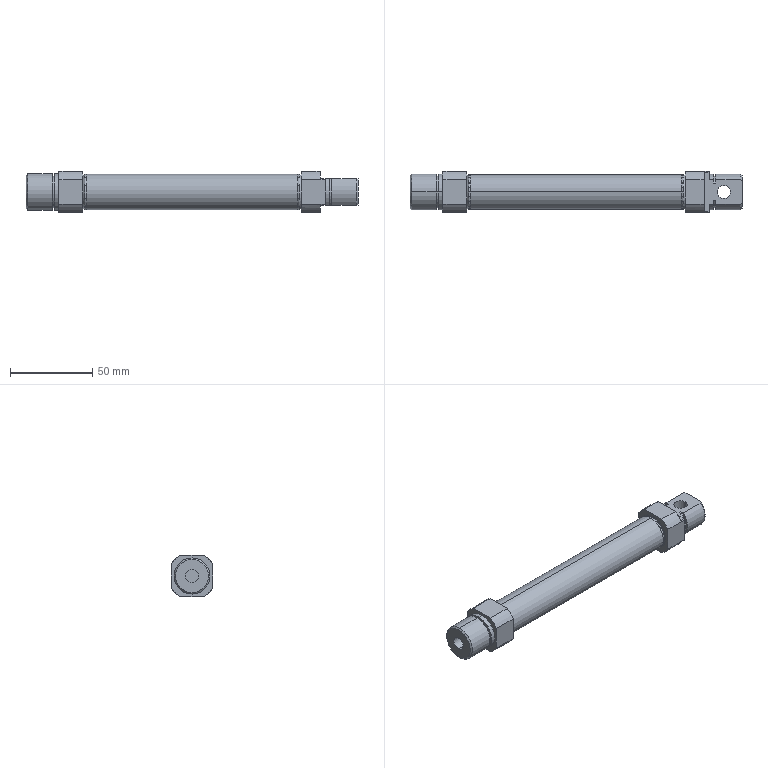Part | SolidWorks | features BaseBody 1 | 1 solid | 88 faces | box 202 x 25 x 25 mm | volume 39660 mm3 | cylinder 36 | plane 32 | cone 16 | torus 4 | commonest cylinder face diameters 22 x8 29 x8 21.4 x6 8 x4 8.566 x4 19.25 x4